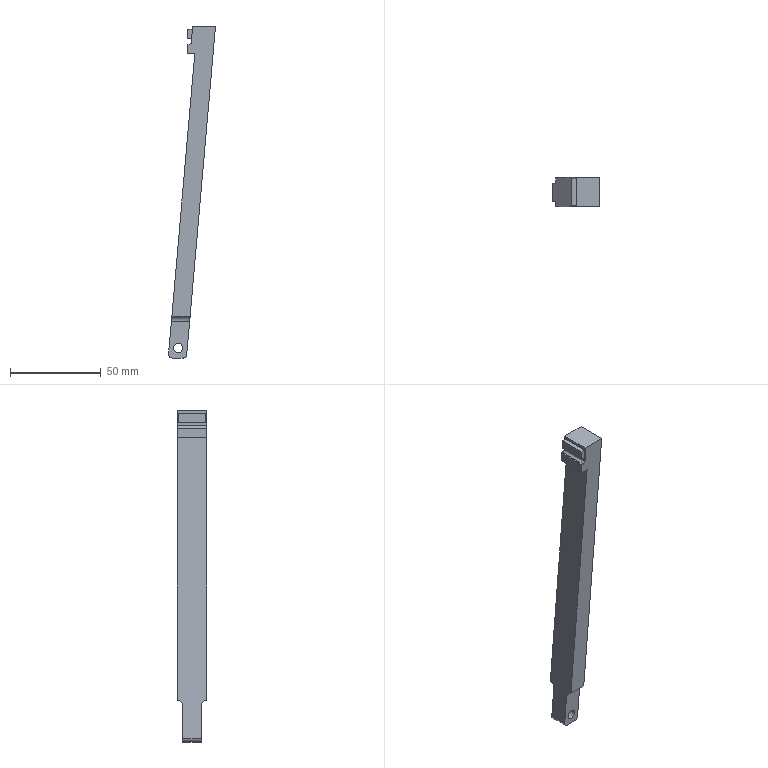Part | STEP file | solid 137 | 1 solid | 38 faces | box 25.825 x 16 x 182.529 mm | volume 28690 mm3 | plane 26 | cylinder 6 | other 6 | commonest cylinder face diameters 4 x2 6 x2 3.016 x1 5 x1